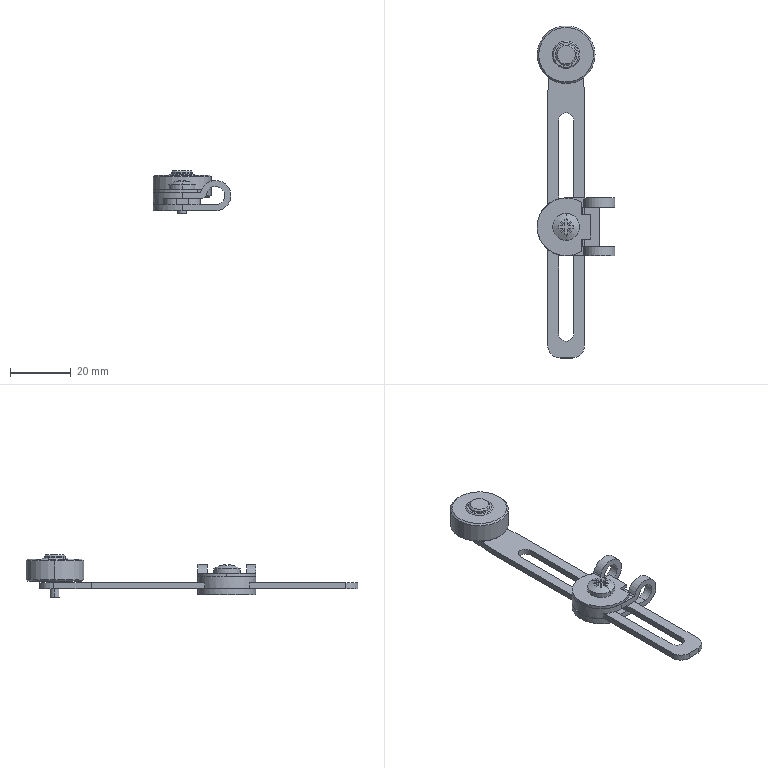Part | STEP file | 2023_07_21_12_39_19_0122 | 1 solid | 128 faces | box 25.5 x 109 x 14 mm | volume 5452 mm3 | plane 77 | cylinder 39 | cone 10 | spline 2 | commonest cylinder face diameters 5 x12 19 x6 10 x5 6 x4 1 x2 3 x2